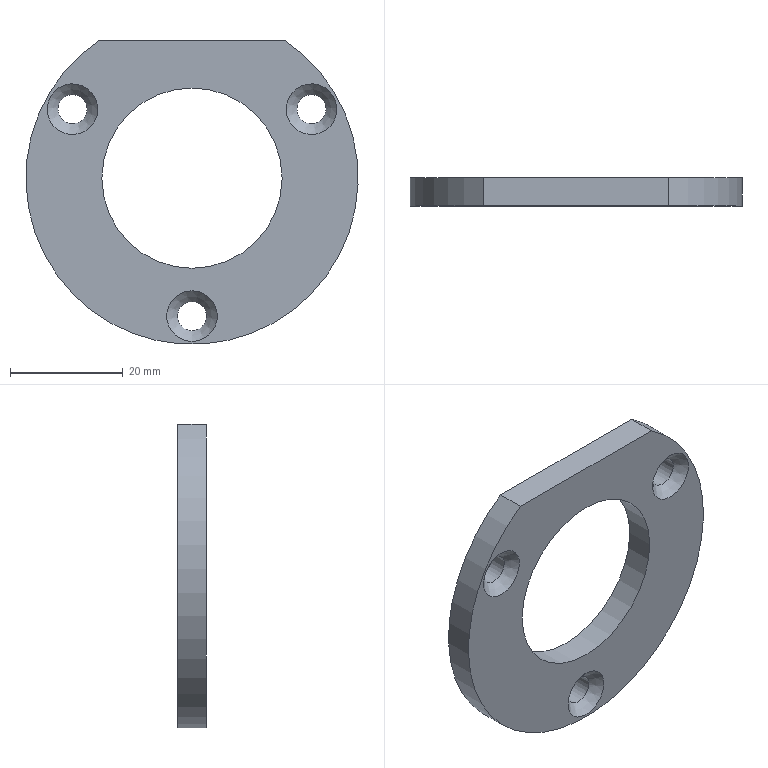Part | STEP file | 冲床-300配套压波_id350_x_t | 1 solid | 11 faces | box 59 x 5 x 54 mm | volume 8662 mm3 | cylinder 5 | cone 3 | plane 3 | commonest cylinder face diameters 5.2 x3 32 x1 59 x1
STEP:
#1=CARTESIAN_POINT('',(1596.531,-102.1,94.05));
#2=VERTEX_POINT('',#1);
#3=CARTESIAN_POINT('',(1598.782,-102.1,92.75));
#4=DIRECTION('',(0.,-1.,0.));
#5=DIRECTION('',(-0.866,0.,0.5));
#6=AXIS2_PLACEMENT_3D('',#3,#4,#5);
#7=CIRCLE('',#6,2.6);
#8=EDGE_CURVE('',#2,#2,#7,.T.);
#9=ORIENTED_EDGE('',*,*,#8,.T.);
#10=EDGE_LOOP('',(#9));
#11=FACE_BOUND('',#10,.T.);
#12=CARTESIAN_POINT('',(1601.034,-99.,91.45));
#13=VERTEX_POINT('',#12);
#14=CARTESIAN_POINT('',(1598.782,-99.,92.75));
#15=DIRECTION('',(0.,-1.,0.));
#16=DIRECTION('',(0.866,0.,-0.5));
#17=AXIS2_PLACEMENT_3D('',#14,#15,#16);
#18=CIRCLE('',#17,2.6);
#19=EDGE_CURVE('',#13,#13,#18,.T.);
#20=ORIENTED_EDGE('',*,*,#19,.F.);
#21=EDGE_LOOP('',(#20));
#22=FACE_BOUND('',#21,.T.);
#23=CARTESIAN_POINT('',(1598.782,494997.324,92.75));
#24=DIRECTION('',(0.,1.,0.));
#25=DIRECTION('',(-0.866,0.,0.5));
#26=AXIS2_PLACEMENT_3D('',#23,#24,#25);
#27=CYLINDRICAL_SURFACE('',#26,2.6);
#28=ADVANCED_FACE('',(#11,#22),#27,.F.);
#29=ORIENTED_EDGE('',*,*,#8,.F.);
#30=EDGE_LOOP('',(#29));
#31=FACE_BOUND('',#30,.T.);
#32=CARTESIAN_POINT('',(1594.885,-104.,95.));
#33=VERTEX_POINT('',#32);
#34=CARTESIAN_POINT('',(1598.782,-104.,92.75));
#35=DIRECTION('',(0.,1.,0.));
#36=DIRECTION('',(-0.866,0.,0.5));
#37=AXIS2_PLACEMENT_3D('',#34,#35,#36);
#38=CIRCLE('',#37,4.5);
#39=EDGE_CURVE('',#33,#33,#38,.T.);
#40=ORIENTED_EDGE('',*,*,#39,.F.);
#41=EDGE_LOOP('',(#40));
#42=FACE_BOUND('',#41,.T.);
#43=CARTESIAN_POINT('',(1598.782,-104.,92.75));
#44=DIRECTION('',(0.,-1.,0.));
#45=DIRECTION('',(0.866,0.,-0.5));
#46=AXIS2_PLACEMENT_3D('',#43,#44,#45);
#47=CONICAL_SURFACE('',#46,4.5,45.);
#48=ADVANCED_FACE('',(#31,#42),#47,.F.);
#49=CARTESIAN_POINT('',(1643.469,-102.1,94.05));
#50=VERTEX_POINT('',#49);
#51=CARTESIAN_POINT('',(1641.218,-102.1,92.75));
#52=DIRECTION('',(0.,-1.,0.));
#53=DIRECTION('',(0.866,0.,0.5));
#54=AXIS2_PLACEMENT_3D('',#51,#52,#53);
#55=CIRCLE('',#54,2.6);
#56=EDGE_CURVE('',#50,#50,#55,.T.);
#57=ORIENTED_EDGE('',*,*,#56,.T.);
#58=EDGE_LOOP('',(#57));
#59=FACE_BOUND('',#58,.T.);
#60=CARTESIAN_POINT('',(1638.966,-99.,91.45));
#61=VERTEX_POINT('',#60);
#62=CARTESIAN_POINT('',(1641.218,-99.,92.75));
#63=DIRECTION('',(0.,-1.,0.));
#64=DIRECTION('',(-0.866,0.,-0.5));
#65=AXIS2_PLACEMENT_3D('',#62,#63,#64);
#66=CIRCLE('',#65,2.6);
#67=EDGE_CURVE('',#61,#61,#66,.T.);
#68=ORIENTED_EDGE('',*,*,#67,.F.);
#69=EDGE_LOOP('',(#68));
#70=FACE_BOUND('',#69,.T.);
#71=CARTESIAN_POINT('',(1641.218,494997.324,92.75));
#72=DIRECTION('',(0.,1.,0.));
#73=DIRECTION('',(0.866,0.,0.5));
#74=AXIS2_PLACEMENT_3D('',#71,#72,#73);
#75=CYLINDRICAL_SURFACE('',#74,2.6);
#76=ADVANCED_FACE('',(#59,#70),#75,.F.);
#77=ORIENTED_EDGE('',*,*,#56,.F.);
#78=EDGE_LOOP('',(#77));
#79=FACE_BOUND('',#78,.T.);
#80=CARTESIAN_POINT('',(1645.115,-104.,95.));
#81=VERTEX_POINT('',#80);
#82=CARTESIAN_POINT('',(1641.218,-104.,92.75));
#83=DIRECTION('',(0.,1.,0.));
#84=DIRECTION('',(0.866,0.,0.5));
#85=AXIS2_PLACEMENT_3D('',#82,#83,#84);
#86=CIRCLE('',#85,4.5);
#87=EDGE_CURVE('',#81,#81,#86,.T.);
#88=ORIENTED_EDGE('',*,*,#87,.F.);
#89=EDGE_LOOP('',(#88));
#90=FACE_BOUND('',#89,.T.);
#91=CARTESIAN_POINT('',(1641.218,-104.,92.75));
#92=DIRECTION('',(0.,-1.,0.));
#93=DIRECTION('',(-0.866,0.,-0.5));
#94=AXIS2_PLACEMENT_3D('',#91,#92,#93);
#95=CONICAL_SURFACE('',#94,4.5,45.);
#96=ADVANCED_FACE('',(#79,#90),#95,.F.);
#97=CARTESIAN_POINT('',(1636.432,-99.,105.));
#98=VERTEX_POINT('',#97);
#99=CARTESIAN_POINT('',(1636.432,-104.,105.));
#100=VERTEX_POINT('',#99);
#101=CARTESIAN_POINT('',(1636.432,-99.,105.));
#102=DIRECTION('',(0.,-1.,0.));
#103=VECTOR('',#102,1.);
#104=LINE('',#101,#103);
#105=EDGE_CURVE('',#98,#100,#104,.T.);
#106=ORIENTED_EDGE('',*,*,#105,.F.);
#107=CARTESIAN_POINT('',(1603.568,-99.,105.));
#108=VERTEX_POINT('',#107);
#109=CARTESIAN_POINT('',(1620.,-99.,105.));
#110=DIRECTION('',(-1.,0.,0.));
#111=VECTOR('',#110,1.);
#112=LINE('',#109,#111);
#113=EDGE_CURVE('',#98,#108,#112,.T.);
#114=ORIENTED_EDGE('',*,*,#113,.T.);
#115=CARTESIAN_POINT('',(1603.568,-104.,105.));
#116=VERTEX_POINT('',#115);
#117=CARTESIAN_POINT('',(1603.568,-99.,105.));
#118=DIRECTION('',(0.,1.,0.));
#119=VECTOR('',#118,1.);
#120=LINE('',#117,#119);
#121=EDGE_CURVE('',#116,#108,#120,.T.);
#122=ORIENTED_EDGE('',*,*,#121,.F.);
#123=CARTESIAN_POINT('',(1620.,-104.,105.));
#124=DIRECTION('',(-1.,0.,0.));
#125=VECTOR('',#124,1.);
#126=LINE('',#123,#125);
#127=EDGE_CURVE('',#100,#116,#126,.T.);
#128=ORIENTED_EDGE('',*,*,#127,.F.);
#129=EDGE_LOOP('',(#106,#114,#122,#128));
#130=FACE_OUTER_BOUND('',#129,.T.);
#131=CARTESIAN_POINT('',(1620.,-104.,105.));
#132=DIRECTION('',(0.,0.,1.));
#133=DIRECTION('',(1.,0.,0.));
#134=AXIS2_PLACEMENT_3D('',#131,#132,#133);
#135=PLANE('',#134);
#136=ADVANCED_FACE('',(#130),#135,.T.);
#137=CARTESIAN_POINT('',(1620.,-104.,80.5));
#138=DIRECTION('',(0.,-1.,0.));
#139=DIRECTION('',(-1.,0.,0.));
#140=AXIS2_PLACEMENT_3D('',#137,#138,#139);
#141=CIRCLE('',#140,29.5);
#142=EDGE_CURVE('',#116,#100,#141,.T.);
#143=ORIENTED_EDGE('',*,*,#142,.F.);
#144=ORIENTED_EDGE('',*,*,#121,.T.);
#145=CARTESIAN_POINT('',(1620.,-99.,80.5));
#146=DIRECTION('',(0.,-1.,0.));
#147=DIRECTION('',(-1.,0.,0.));
#148=AXIS2_PLACEMENT_3D('',#145,#146,#147);
#149=CIRCLE('',#148,29.5);
#150=EDGE_CURVE('',#108,#98,#149,.T.);
#151=ORIENTED_EDGE('',*,*,#150,.T.);
#152=ORIENTED_EDGE('',*,*,#105,.T.);
#153=EDGE_LOOP('',(#143,#144,#151,#152));
#154=FACE_OUTER_BOUND('',#153,.T.);
#155=CARTESIAN_POINT('',(1620.,-99.,80.5));
#156=DIRECTION('',(0.,-1.,0.));
#157=DIRECTION('',(0.,0.,1.));
#158=AXIS2_PLACEMENT_3D('',#155,#156,#157);
#159=CYLINDRICAL_SURFACE('',#158,29.5);
#160=ADVANCED_FACE('',(#154),#159,.T.);
#161=ORIENTED_EDGE('',*,*,#19,.T.);
#162=EDGE_LOOP('',(#161));
#163=FACE_BOUND('',#162,.T.);
#164=ORIENTED_EDGE('',*,*,#67,.T.);
#165=EDGE_LOOP('',(#164));
#166=FACE_BOUND('',#165,.T.);
#167=CARTESIAN_POINT('',(1620.,-99.,58.6));
#168=VERTEX_POINT('',#167);
#169=CARTESIAN_POINT('',(1620.,-99.,56.));
#170=DIRECTION('',(0.,-1.,0.));
#171=DIRECTION('',(0.,0.,1.));
#172=AXIS2_PLACEMENT_3D('',#169,#170,#171);
#173=CIRCLE('',#172,2.6);
#174=EDGE_CURVE('',#168,#168,#173,.T.);
#175=ORIENTED_EDGE('',*,*,#174,.T.);
#176=EDGE_LOOP('',(#175));
#177=FACE_BOUND('',#176,.T.);
#178=CARTESIAN_POINT('',(1620.,-99.,64.5));
#179=VERTEX_POINT('',#178);
#180=CARTESIAN_POINT('',(1620.,-99.,80.5));
#181=DIRECTION('',(0.,-1.,0.));
#182=DIRECTION('',(0.,0.,-1.));
#183=AXIS2_PLACEMENT_3D('',#180,#181,#182);
#184=CIRCLE('',#183,16.);
#185=EDGE_CURVE('',#179,#179,#184,.T.);
#186=ORIENTED_EDGE('',*,*,#185,.T.);
#187=EDGE_LOOP('',(#186));
#188=FACE_BOUND('',#187,.T.);
#189=ORIENTED_EDGE('',*,*,#113,.F.);
#190=ORIENTED_EDGE('',*,*,#150,.F.);
#191=EDGE_LOOP('',(#189,#190));
#192=FACE_BOUND('',#191,.T.);
#193=CARTESIAN_POINT('',(1620.,-99.,80.5));
#194=DIRECTION('',(0.,-1.,0.));
#195=DIRECTION('',(0.,0.,1.));
#196=AXIS2_PLACEMENT_3D('',#193,#194,#195);
#197=PLANE('',#196);
#198=ADVANCED_FACE('',(#163,#166,#177,#188,#192),#197,.F.);
#199=ORIENTED_EDGE('',*,*,#39,.T.);
#200=EDGE_LOOP('',(#199));
#201=FACE_BOUND('',#200,.T.);
#202=ORIENTED_EDGE('',*,*,#87,.T.);
#203=EDGE_LOOP('',(#202));
#204=FACE_BOUND('',#203,.T.);
#205=CARTESIAN_POINT('',(1620.,-104.,51.5));
#206=VERTEX_POINT('',#205);
#207=CARTESIAN_POINT('',(1620.,-104.,56.));
#208=DIRECTION('',(0.,1.,0.));
#209=DIRECTION('',(0.,0.,-1.));
#210=AXIS2_PLACEMENT_3D('',#207,#208,#209);
#211=CIRCLE('',#210,4.5);
#212=EDGE_CURVE('',#206,#206,#211,.T.);
#213=ORIENTED_EDGE('',*,*,#212,.T.);
#214=EDGE_LOOP('',(#213));
#215=FACE_BOUND('',#214,.T.);
#216=CARTESIAN_POINT('',(1620.,-104.,64.5));
#217=VERTEX_POINT('',#216);
#218=CARTESIAN_POINT('',(1620.,-104.,80.5));
#219=DIRECTION('',(0.,-1.,0.));
#220=DIRECTION('',(0.,0.,-1.));
#221=AXIS2_PLACEMENT_3D('',#218,#219,#220);
#222=CIRCLE('',#221,16.);
#223=EDGE_CURVE('',#217,#217,#222,.T.);
#224=ORIENTED_EDGE('',*,*,#223,.F.);
#225=EDGE_LOOP('',(#224));
#226=FACE_BOUND('',#225,.T.);
#227=ORIENTED_EDGE('',*,*,#142,.T.);
#228=ORIENTED_EDGE('',*,*,#127,.T.);
#229=EDGE_LOOP('',(#227,#228));
#230=FACE_BOUND('',#229,.T.);
#231=CARTESIAN_POINT('',(1620.,-104.,80.5));
#232=DIRECTION('',(0.,-1.,0.));
#233=DIRECTION('',(0.,0.,1.));
#234=AXIS2_PLACEMENT_3D('',#231,#232,#233);
#235=PLANE('',#234);
#236=ADVANCED_FACE('',(#201,#204,#215,#226,#230),#235,.T.);
#237=ORIENTED_EDGE('',*,*,#223,.T.);
#238=EDGE_LOOP('',(#237));
#239=FACE_BOUND('',#238,.T.);
#240=ORIENTED_EDGE('',*,*,#185,.F.);
#241=EDGE_LOOP('',(#240));
#242=FACE_BOUND('',#241,.T.);
#243=CARTESIAN_POINT('',(1620.,-75.,80.5));
#244=DIRECTION('',(0.,-1.,0.));
#245=DIRECTION('',(-1.,0.,0.));
#246=AXIS2_PLACEMENT_3D('',#243,#244,#245);
#247=CYLINDRICAL_SURFACE('',#246,16.);
#248=ADVANCED_FACE('',(#239,#242),#247,.F.);
#249=CARTESIAN_POINT('',(1620.,-102.1,53.4));
#250=VERTEX_POINT('',#249);
#251=CARTESIAN_POINT('',(1620.,-102.1,56.));
#252=DIRECTION('',(0.,-1.,0.));
#253=DIRECTION('',(0.,0.,-1.));
#254=AXIS2_PLACEMENT_3D('',#251,#252,#253);
#255=CIRCLE('',#254,2.6);
#256=EDGE_CURVE('',#250,#250,#255,.T.);
#257=ORIENTED_EDGE('',*,*,#256,.T.);
#258=EDGE_LOOP('',(#257));
#259=FACE_BOUND('',#258,.T.);
#260=ORIENTED_EDGE('',*,*,#174,.F.);
#261=EDGE_LOOP('',(#260));
#262=FACE_BOUND('',#261,.T.);
#263=CARTESIAN_POINT('',(1620.,494997.324,56.));
#264=DIRECTION('',(0.,1.,0.));
#265=DIRECTION('',(0.,0.,-1.));
#266=AXIS2_PLACEMENT_3D('',#263,#264,#265);
#267=CYLINDRICAL_SURFACE('',#266,2.6);
#268=ADVANCED_FACE('',(#259,#262),#267,.F.);
#269=ORIENTED_EDGE('',*,*,#256,.F.);
#270=EDGE_LOOP('',(#269));
#271=FACE_BOUND('',#270,.T.);
#272=ORIENTED_EDGE('',*,*,#212,.F.);
#273=EDGE_LOOP('',(#272));
#274=FACE_BOUND('',#273,.T.);
#275=CARTESIAN_POINT('',(1620.,-104.,56.));
#276=DIRECTION('',(0.,-1.,0.));
#277=DIRECTION('',(0.,0.,1.));
#278=AXIS2_PLACEMENT_3D('',#275,#276,#277);
#279=CONICAL_SURFACE('',#278,4.5,45.);
#280=ADVANCED_FACE('',(#271,#274),#279,.F.);
#281=CLOSED_SHELL('',(#28,#48,#76,#96,#136,#160,#198,#236,#248,#268,#280));
#282=MANIFOLD_SOLID_BREP('',#281);
#283=(LENGTH_UNIT()NAMED_UNIT(*)SI_UNIT(.MILLI.,.METRE.));
#284=UNCERTAINTY_MEASURE_WITH_UNIT(LENGTH_MEASURE(0.00002),#283,'','');
#285=(NAMED_UNIT(*)PLANE_ANGLE_UNIT()SI_UNIT($,.RADIAN.));
#286=PLANE_ANGLE_MEASURE_WITH_UNIT(PLANE_ANGLE_MEASURE(0.01745),#285);
#287=DIMENSIONAL_EXPONENTS(0.,0.,0.,0.,0.,0.,0.);
#288=(CONVERSION_BASED_UNIT('DEGREE',#286)NAMED_UNIT(#287)PLANE_ANGLE_UNIT());
#289=(NAMED_UNIT(*)SI_UNIT($,.STERADIAN.)SOLID_ANGLE_UNIT());
#290=(GEOMETRIC_REPRESENTATION_CONTEXT(3)GLOBAL_UNCERTAINTY_ASSIGNED_CONTEXT((#284))GLOBAL_UNIT_ASSIGNED_CONTEXT((#283,#288,#289))REPRESENTATION_CONTEXT('',''));
#291=ADVANCED_BREP_SHAPE_REPRESENTATION('',(#282),#290);